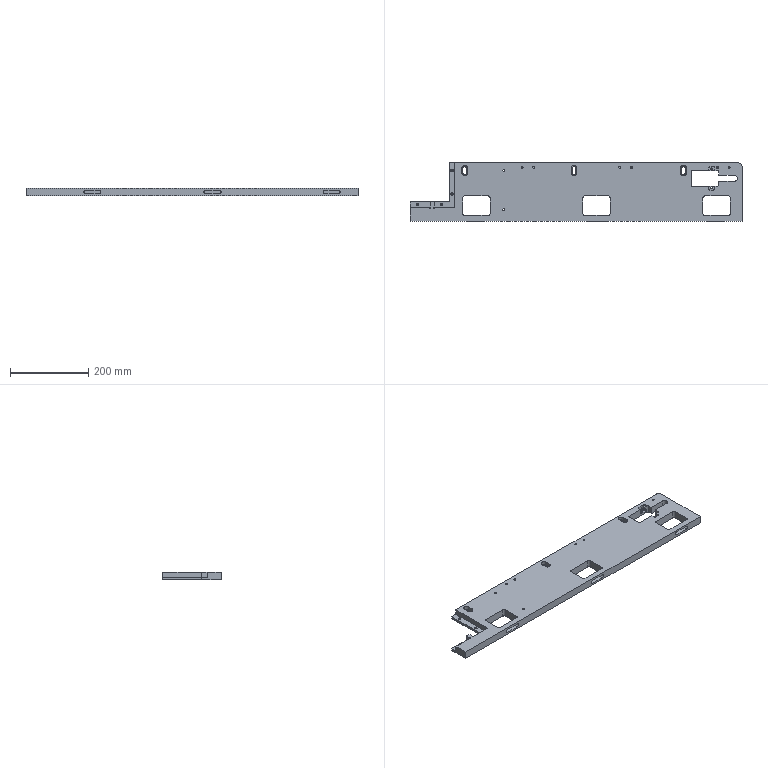Part | SolidWorks | features HoleWzd 7, ICE 6, Fillet 4, Cut 1, Extrusion 1, LPattern 1 | 1 solid | 192 faces | box 850 x 150 x 20 mm | volume 1984995 mm3 | cylinder 92 | plane 63 | cone 37 | commonest cylinder face diameters 5 x47 9 x12 10 x12 6 x9 15 x6 3 x3